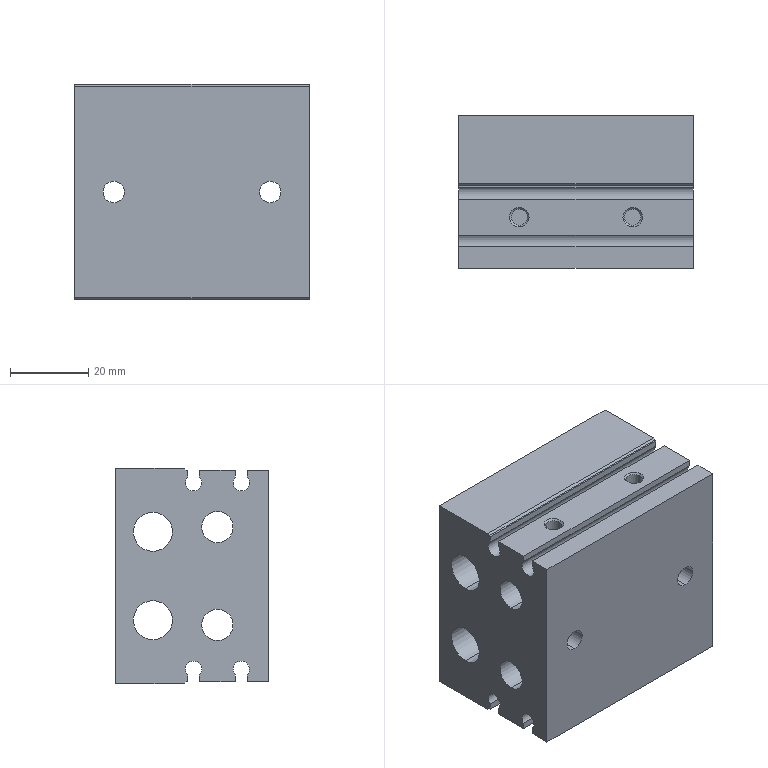Part | SolidWorks | features BaseBody 1 | 1 solid | 92 faces | box 60 x 39 x 55 mm | volume 104466 mm3 | cylinder 41 | plane 35 | cone 16 | commonest cylinder face diameters 4.134 x16 4.2 x6 3 x5 5.5 x4 8 x4 10 x4